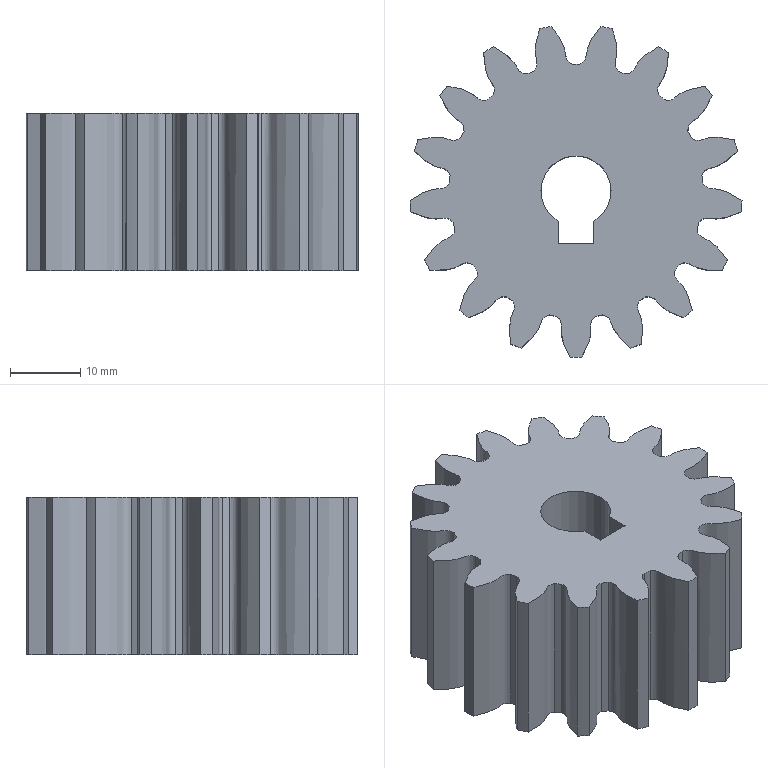Part | SolidWorks | features Attribute 3, ICE 2, CirPattern 1, Cut 1, Extrusion 1, RefAxis 1, Scale 1 | 1 solid | 76 faces | box 47.423 x 47.235 x 22.5 mm | volume 29237 mm3 | cylinder 37 | spline 34 | plane 5 | commonest cylinder face diameters 36.25 x17 47.5 x17 10 x3